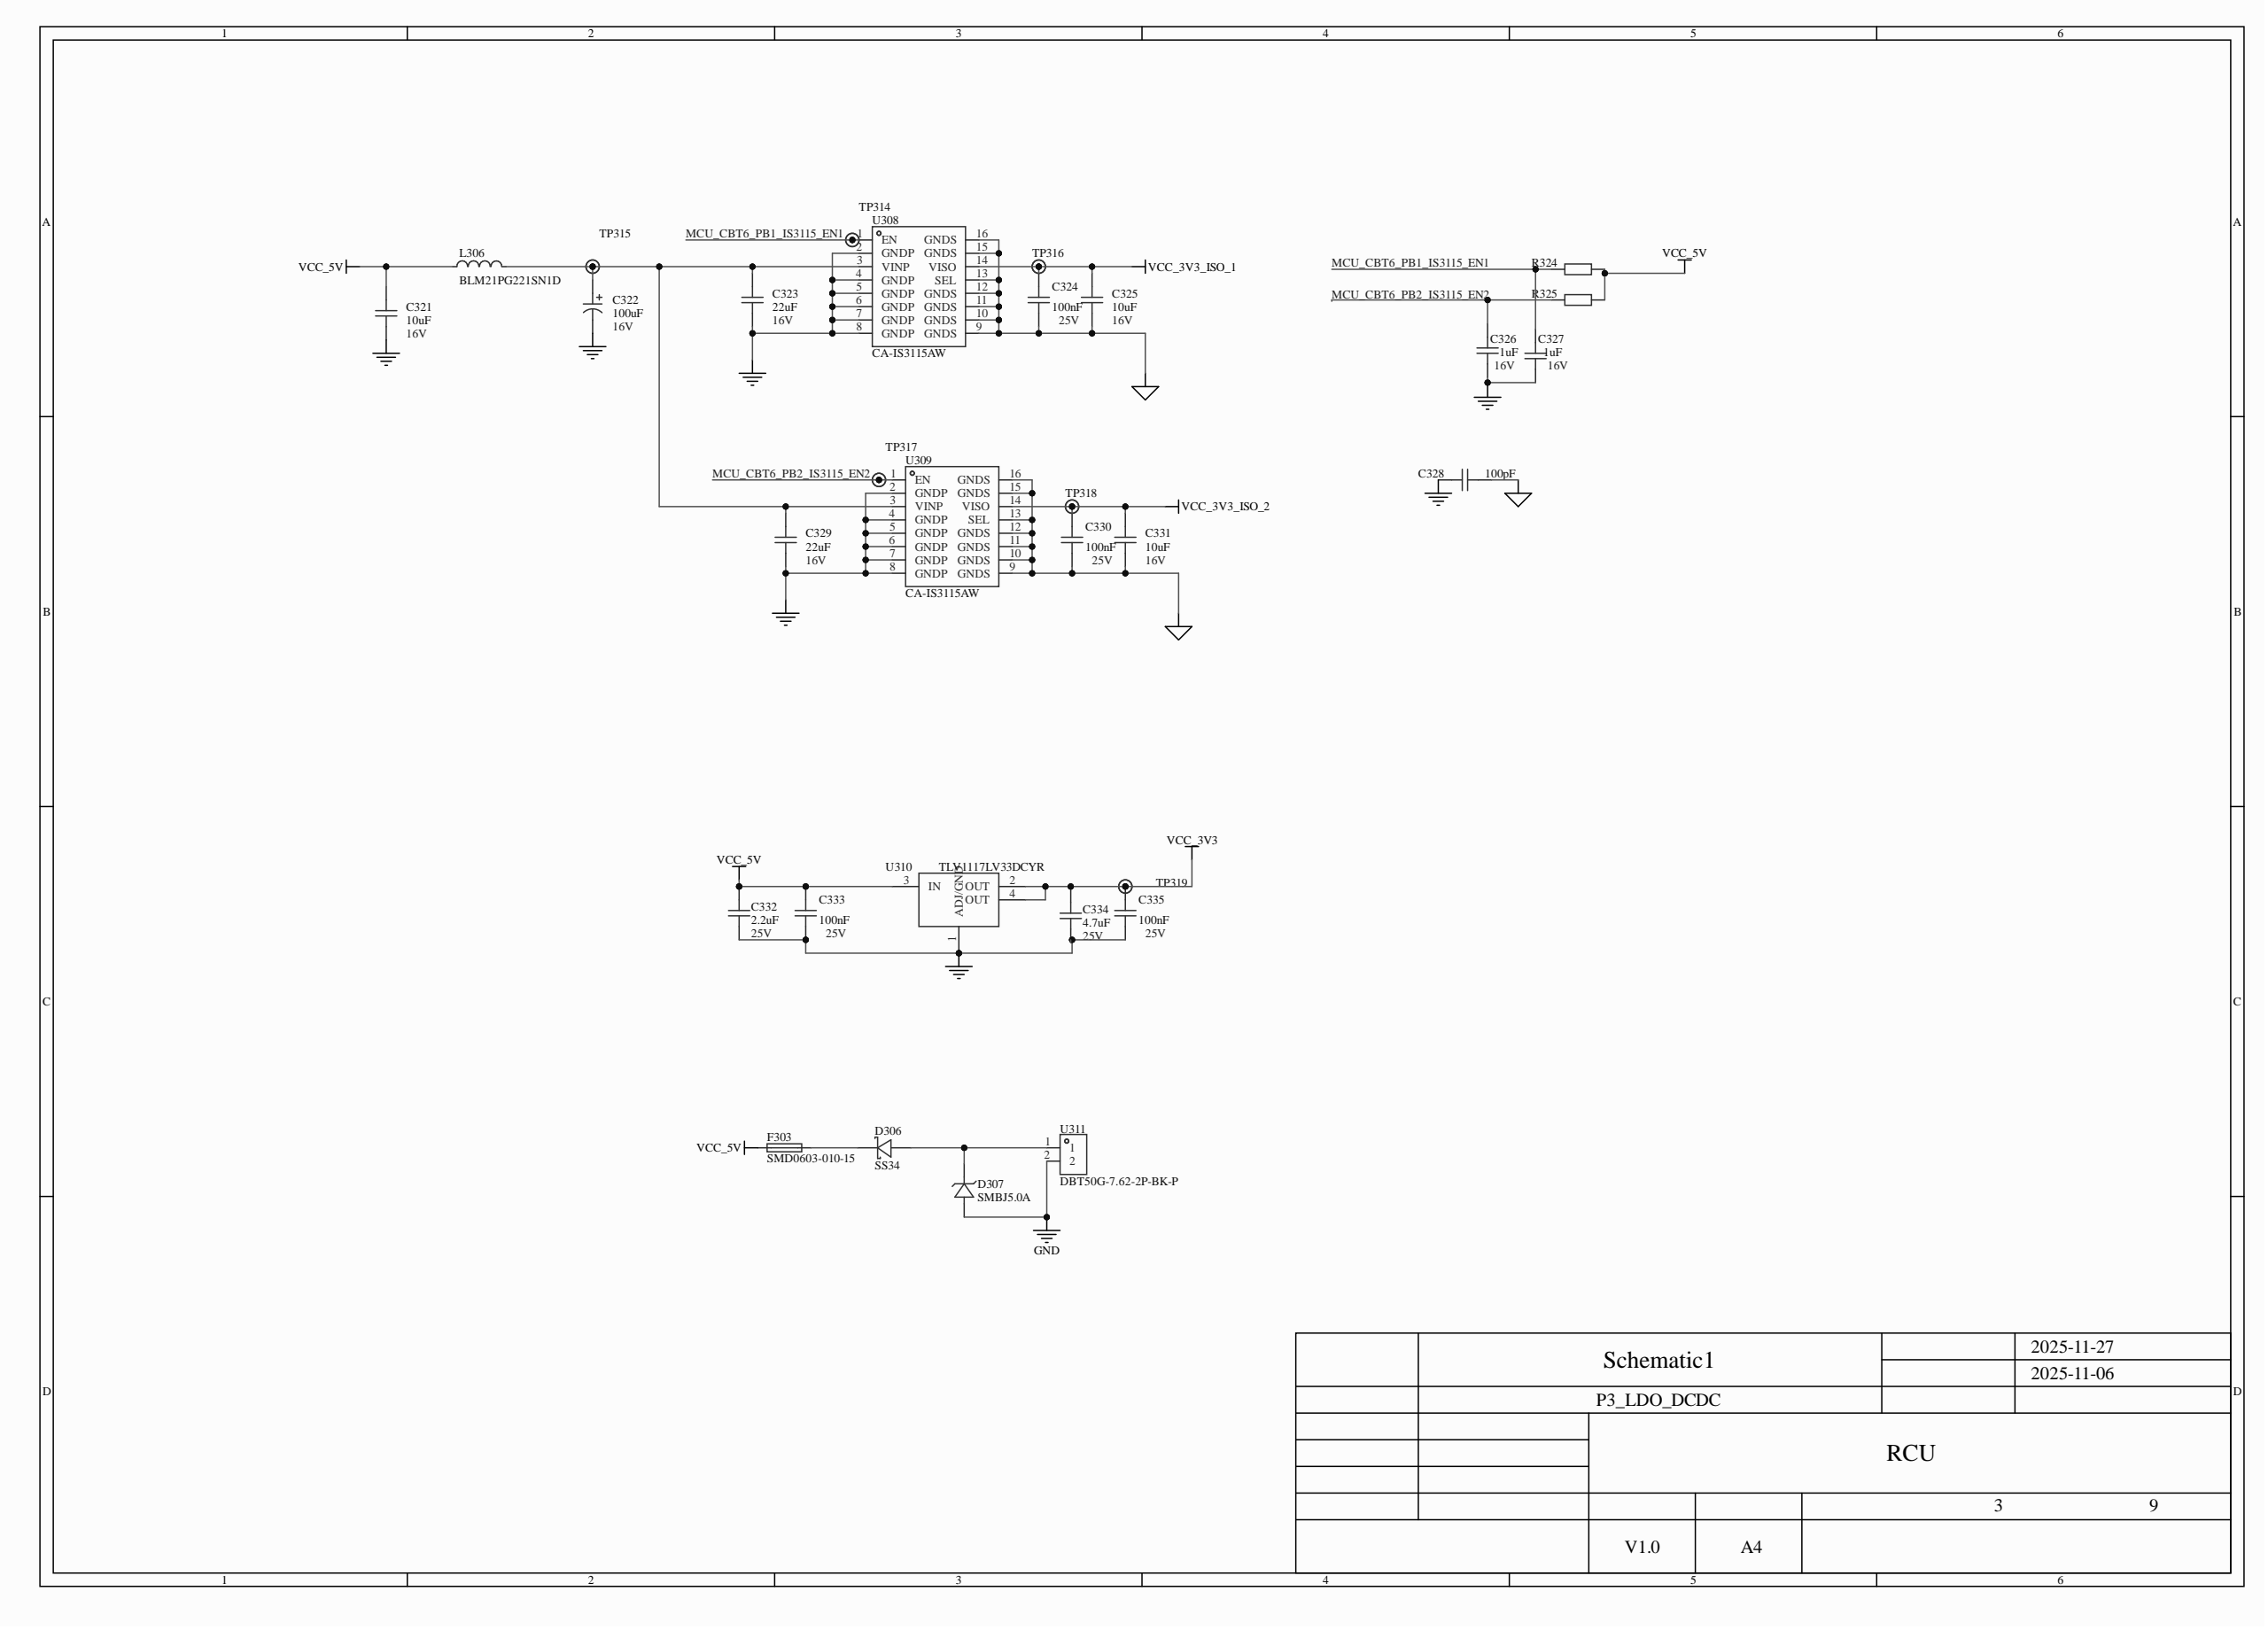Circuit board | Altium Designer | 424 parts | 202 nets | one sheet of the schematic
Parts on this sheet (reference | value | footprint):
C321 | 10uF | C0805
C322 | 100uF | CAP-SMD_BD6.3-L6.6-W6.6-LS7.2-FD
C323 | 22uF | C0603
C324 | 100nF | C0603
C325 | 10uF | C0805
C326 | 1uF | C0603
C327 | 1uF | C0603
C328 | 100pF | CAP-TH_L7.0-W4.0-P10.00-D0.6
C329 | 22uF | C0603
C330 | 100nF | C0603
C331 | 10uF | C0805
C332 | 2.2uF | C0603
C333 | 100nF | C0603
C334 | 4.7uF | C0603
C335 | 100nF | C0603
D306 | SS34 | SMC_L6.9-W5.9-LS7.9-RD
D307 | SMBJ5.0A | SMB_L4.6-W3.6-LS5.4-RD
F303 | SMD0603-010-15 | F0603
L306 | BLM21PG221SN1D | L0805
R324 | R0603
R325 | R0603
TP314 | Test-Point-0.5mm
TP315 | Test-Point-0.5mm
TP316 | Test-Point-0.5mm
TP317 | Test-Point-0.5mm
TP318 | Test-Point-0.5mm
TP319 | Test-Point-0.5mm
U308 | CA-IS3115AW | SOIC-16_L10.3-W7.5-P1.27-LS10.3-BL
U309 | CA-IS3115AW | SOIC-16_L10.3-W7.5-P1.27-LS10.3-BL
U310 | TLV1117LV33DCYR | SOT-223_L6.7-W3.5-P2.30-BR
U311 | DBT50G-7.62-2P-BK-P | CONN-TH_2P-P7.62_L15.2-W16.7-EX4.2
Nets of these parts (net: part-pin ...):
VCC_5V: C321-2 C332-2 C333-1 F303-1 L306-1 R324-2 R325-2 U310-3
VCC_3V3_ISO_2: C330-1 C331-2 TP318-1 U309-14
VCC_3V3_ISO_1: C324-1 C325-2 TP316-1 U308-14
VCC_3V3: C334-2 C335-1 TP319-1 U310-2 U310-4
PGND: C324-2 C325-1 C328-2 C330-2 C331-1 U308-9 U308-10 U308-11 U308-12 U308-13 U308-15 U308-16 U309-9 U309-10 U309-11 U309-12 U309-13 U309-15 U309-16
NetD306_2: D306-2 D307-1 U311-1
NetD306_1: D306-1 F303-2
NetC322_1: C322-1 C323-2 C329-2 L306-2 TP315-1 U308-3 U309-3
MCU_CBT6_PB2_IS3115_EN2: C326-2 R325-1 TP317-1 U309-1
MCU_CBT6_PB1_IS3115_EN1: C327-2 R324-1 TP314-1 U308-1
GND: C321-1 C322-2 C323-1 C326-1 C327-1 C328-1 C329-1 C332-1 C333-2 C334-1 C335-2 D307-2 U308-2 U308-4 U308-5 U308-6 U308-7 U308-8 U309-2 U309-4 U309-5 U309-6 U309-7 U309-8 U310-1 U311-2